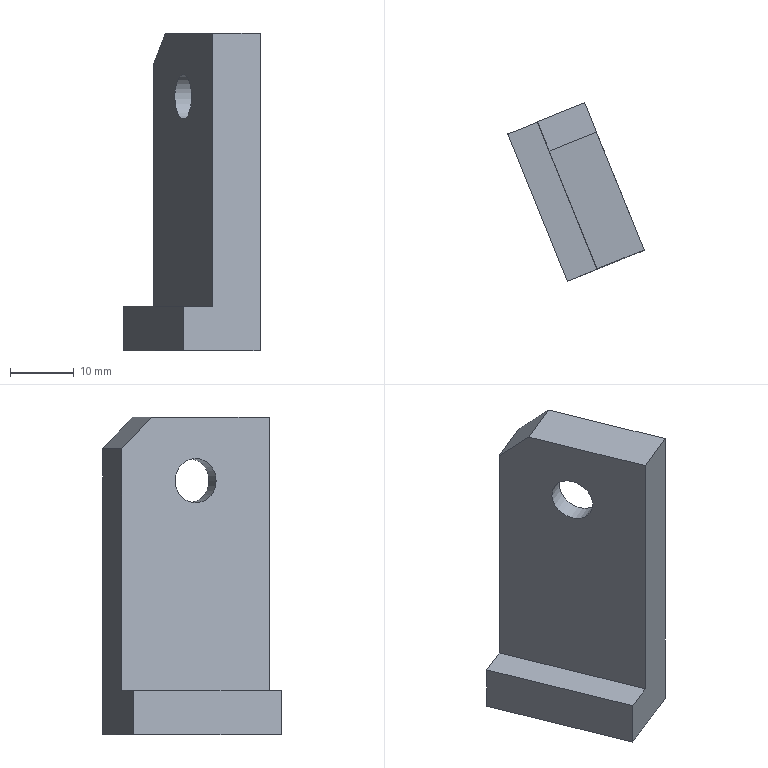Part | NX | features solid 2 | 1 solid | 12 faces | box 21.419 x 28.049 x 50 mm | volume 9656 mm3 | plane 10 | spline 2
STEP:
#1=CARTESIAN_POINT('',(-700.084,400.509,62.979));
#2=VERTEX_POINT('',#1);
#3=CARTESIAN_POINT('',(-699.783,399.764,61.255));
#4=CARTESIAN_POINT('',(-700.385,401.254,64.703));
#5=CARTESIAN_POINT('',(-701.18,403.223,65.476));
#6=CARTESIAN_POINT('',(-702.472,406.42,63.868));
#7=CARTESIAN_POINT('',(-702.761,407.136,61.745));
#8=CARTESIAN_POINT('',(-702.159,405.646,58.297));
#9=CARTESIAN_POINT('',(-701.364,403.677,57.524));
#10=CARTESIAN_POINT('',(-700.072,400.48,59.132));
#11=CARTESIAN_POINT('',(-699.783,399.764,61.255));
#12=CARTESIAN_POINT('',(-700.385,401.254,64.703));
#13=B_SPLINE_CURVE_WITH_KNOTS('',3,(#3,#4,#5,#6,#7,#8,#9,#10,#11,#12),.UNSPECIFIED.,.T.,.F.,(2,2,2,2,2,2,2),(-0.25,0.,0.25,0.5,0.75,1.,1.25),.UNSPECIFIED.);
#14=EDGE_CURVE('',#2,#2,#13,.T.);
#15=ORIENTED_EDGE('',*,*,#14,.F.);
#16=EDGE_LOOP('',(#15));
#17=FACE_BOUND('',#16,.T.);
#18=CARTESIAN_POINT('',(-705.955,415.04,28.5));
#19=VERTEX_POINT('',#18);
#20=CARTESIAN_POINT('',(-696.589,391.86,28.5));
#21=VERTEX_POINT('',#20);
#22=CARTESIAN_POINT('',(-696.589,391.86,28.5));
#23=DIRECTION('',(0.3746,-0.9272,0.000000023));
#24=VECTOR('',#23,1000.);
#25=LINE('',#22,#24);
#26=EDGE_CURVE('',#19,#21,#25,.T.);
#27=ORIENTED_EDGE('',*,*,#26,.T.);
#28=CARTESIAN_POINT('',(-696.589,391.86,71.5));
#29=VERTEX_POINT('',#28);
#30=CARTESIAN_POINT('',(-696.589,391.86,21.5));
#31=DIRECTION('',(0.,0.,1.));
#32=VECTOR('',#31,1000.);
#33=LINE('',#30,#32);
#34=EDGE_CURVE('',#21,#29,#33,.T.);
#35=ORIENTED_EDGE('',*,*,#34,.T.);
#36=CARTESIAN_POINT('',(-704.082,410.404,71.5));
#37=VERTEX_POINT('',#36);
#38=CARTESIAN_POINT('',(-696.589,391.86,71.5));
#39=DIRECTION('',(-0.3746,0.9272,0.));
#40=VECTOR('',#39,1000.);
#41=LINE('',#38,#40);
#42=EDGE_CURVE('',#29,#37,#41,.T.);
#43=ORIENTED_EDGE('',*,*,#42,.T.);
#44=CARTESIAN_POINT('',(-705.955,415.04,66.5));
#45=VERTEX_POINT('',#44);
#46=CARTESIAN_POINT('',(-705.955,415.04,66.5));
#47=DIRECTION('',(0.2649,-0.6556,0.7071));
#48=VECTOR('',#47,1000.);
#49=LINE('',#46,#48);
#50=EDGE_CURVE('',#45,#37,#49,.T.);
#51=ORIENTED_EDGE('',*,*,#50,.F.);
#52=CARTESIAN_POINT('',(-705.955,415.04,51.5));
#53=DIRECTION('',(0.,0.,1.));
#54=VECTOR('',#53,1000.);
#55=LINE('',#52,#54);
#56=EDGE_CURVE('',#19,#45,#55,.T.);
#57=ORIENTED_EDGE('',*,*,#56,.F.);
#58=EDGE_LOOP('',(#27,#35,#43,#51,#57));
#59=FACE_BOUND('',#58,.T.);
#60=CARTESIAN_POINT('',(-696.589,391.86,91.5));
#61=DIRECTION('',(0.9272,0.3746,0.));
#62=DIRECTION('',(0.3244,-0.803,0.5));
#63=AXIS2_PLACEMENT_3D('',#60,#61,#62);
#64=PLANE('',#63);
#65=ADVANCED_FACE('',(#17,#59),#64,.F.);
#66=CARTESIAN_POINT('',(-698.537,418.037,66.5));
#67=VERTEX_POINT('',#66);
#68=CARTESIAN_POINT('',(-696.664,413.401,71.5));
#69=VERTEX_POINT('',#68);
#70=CARTESIAN_POINT('',(-698.537,418.037,66.5));
#71=DIRECTION('',(0.2649,-0.6556,0.7071));
#72=VECTOR('',#71,1000.);
#73=LINE('',#70,#72);
#74=EDGE_CURVE('',#67,#69,#73,.T.);
#75=ORIENTED_EDGE('',*,*,#74,.F.);
#76=CARTESIAN_POINT('',(-705.955,415.04,66.5));
#77=DIRECTION('',(0.9272,0.3746,0.));
#78=VECTOR('',#77,1000.);
#79=LINE('',#76,#78);
#80=EDGE_CURVE('',#45,#67,#79,.T.);
#81=ORIENTED_EDGE('',*,*,#80,.F.);
#82=ORIENTED_EDGE('',*,*,#50,.T.);
#83=CARTESIAN_POINT('',(-704.082,410.404,71.5));
#84=DIRECTION('',(0.9272,0.3746,0.));
#85=VECTOR('',#84,1000.);
#86=LINE('',#83,#85);
#87=EDGE_CURVE('',#37,#69,#86,.T.);
#88=ORIENTED_EDGE('',*,*,#87,.T.);
#89=EDGE_LOOP('',(#75,#81,#82,#88));
#90=FACE_BOUND('',#89,.T.);
#91=CARTESIAN_POINT('',(-705.955,415.04,66.5));
#92=DIRECTION('',(0.2649,-0.6556,-0.7071));
#93=DIRECTION('',(0.2649,-0.6556,0.7071));
#94=AXIS2_PLACEMENT_3D('',#91,#92,#93);
#95=PLANE('',#94);
#96=ADVANCED_FACE('',(#90),#95,.F.);
#97=CARTESIAN_POINT('',(-689.172,394.857,71.5));
#98=VERTEX_POINT('',#97);
#99=CARTESIAN_POINT('',(-689.172,394.857,71.5));
#100=DIRECTION('',(-0.3746,0.9272,0.));
#101=VECTOR('',#100,1000.);
#102=LINE('',#99,#101);
#103=EDGE_CURVE('',#98,#69,#102,.T.);
#104=ORIENTED_EDGE('',*,*,#103,.T.);
#105=ORIENTED_EDGE('',*,*,#87,.F.);
#106=ORIENTED_EDGE('',*,*,#42,.F.);
#107=CARTESIAN_POINT('',(-696.589,391.86,71.5));
#108=DIRECTION('',(0.9272,0.3746,0.));
#109=VECTOR('',#108,1000.);
#110=LINE('',#107,#109);
#111=EDGE_CURVE('',#29,#98,#110,.T.);
#112=ORIENTED_EDGE('',*,*,#111,.T.);
#113=EDGE_LOOP('',(#104,#105,#106,#112));
#114=FACE_BOUND('',#113,.T.);
#115=CARTESIAN_POINT('',(-696.589,391.86,71.5));
#116=DIRECTION('',(0.,0.,1.));
#117=DIRECTION('',(-0.3746,0.9272,0.));
#118=AXIS2_PLACEMENT_3D('',#115,#116,#117);
#119=PLANE('',#118);
#120=ADVANCED_FACE('',(#114),#119,.T.);
#121=CARTESIAN_POINT('',(-689.172,394.857,21.5));
#122=VERTEX_POINT('',#121);
#123=CARTESIAN_POINT('',(-689.172,394.857,21.5));
#124=DIRECTION('',(0.,0.,1.));
#125=VECTOR('',#124,1000.);
#126=LINE('',#123,#125);
#127=EDGE_CURVE('',#122,#98,#126,.T.);
#128=ORIENTED_EDGE('',*,*,#127,.T.);
#129=ORIENTED_EDGE('',*,*,#111,.F.);
#130=ORIENTED_EDGE('',*,*,#34,.F.);
#131=CARTESIAN_POINT('',(-701.225,389.987,28.5));
#132=VERTEX_POINT('',#131);
#133=CARTESIAN_POINT('',(-701.225,389.987,28.5));
#134=DIRECTION('',(0.9272,0.3746,0.));
#135=VECTOR('',#134,1000.);
#136=LINE('',#133,#135);
#137=EDGE_CURVE('',#132,#21,#136,.T.);
#138=ORIENTED_EDGE('',*,*,#137,.F.);
#139=CARTESIAN_POINT('',(-701.225,389.987,21.5));
#140=VERTEX_POINT('',#139);
#141=CARTESIAN_POINT('',(-701.225,389.987,31.5));
#142=DIRECTION('',(0.,0.,-1.));
#143=VECTOR('',#142,1000.);
#144=LINE('',#141,#143);
#145=EDGE_CURVE('',#132,#140,#144,.T.);
#146=ORIENTED_EDGE('',*,*,#145,.T.);
#147=CARTESIAN_POINT('',(-696.589,391.86,21.5));
#148=DIRECTION('',(0.9272,0.3746,0.));
#149=VECTOR('',#148,1000.);
#150=LINE('',#147,#149);
#151=EDGE_CURVE('',#140,#122,#150,.T.);
#152=ORIENTED_EDGE('',*,*,#151,.T.);
#153=EDGE_LOOP('',(#128,#129,#130,#138,#146,#152));
#154=FACE_BOUND('',#153,.T.);
#155=CARTESIAN_POINT('',(-696.589,391.86,21.5));
#156=DIRECTION('',(0.3746,-0.9272,0.));
#157=DIRECTION('',(0.,0.,1.));
#158=AXIS2_PLACEMENT_3D('',#155,#156,#157);
#159=PLANE('',#158);
#160=ADVANCED_FACE('',(#154),#159,.T.);
#161=CARTESIAN_POINT('',(-698.537,418.037,21.5));
#162=VERTEX_POINT('',#161);
#163=CARTESIAN_POINT('',(-698.537,418.037,21.5));
#164=DIRECTION('',(0.3746,-0.9272,0.));
#165=VECTOR('',#164,1000.);
#166=LINE('',#163,#165);
#167=EDGE_CURVE('',#162,#122,#166,.T.);
#168=ORIENTED_EDGE('',*,*,#167,.T.);
#169=ORIENTED_EDGE('',*,*,#151,.F.);
#170=CARTESIAN_POINT('',(-710.591,413.167,21.5));
#171=VERTEX_POINT('',#170);
#172=CARTESIAN_POINT('',(-710.591,413.167,21.5));
#173=DIRECTION('',(0.3746,-0.9272,0.));
#174=VECTOR('',#173,1000.);
#175=LINE('',#172,#174);
#176=EDGE_CURVE('',#171,#140,#175,.T.);
#177=ORIENTED_EDGE('',*,*,#176,.F.);
#178=CARTESIAN_POINT('',(-705.955,415.04,21.5));
#179=DIRECTION('',(0.9272,0.3746,0.));
#180=VECTOR('',#179,1000.);
#181=LINE('',#178,#180);
#182=EDGE_CURVE('',#171,#162,#181,.T.);
#183=ORIENTED_EDGE('',*,*,#182,.T.);
#184=EDGE_LOOP('',(#168,#169,#177,#183));
#185=FACE_BOUND('',#184,.T.);
#186=CARTESIAN_POINT('',(-705.955,415.04,21.5));
#187=DIRECTION('',(0.,0.,-1.));
#188=DIRECTION('',(0.3746,-0.9272,0.));
#189=AXIS2_PLACEMENT_3D('',#186,#187,#188);
#190=PLANE('',#189);
#191=ADVANCED_FACE('',(#185),#190,.T.);
#192=CARTESIAN_POINT('',(-698.537,418.037,51.5));
#193=DIRECTION('',(0.,0.,1.));
#194=VECTOR('',#193,1000.);
#195=LINE('',#192,#194);
#196=EDGE_CURVE('',#162,#67,#195,.T.);
#197=ORIENTED_EDGE('',*,*,#196,.F.);
#198=ORIENTED_EDGE('',*,*,#182,.F.);
#199=CARTESIAN_POINT('',(-710.591,413.167,28.5));
#200=VERTEX_POINT('',#199);
#201=CARTESIAN_POINT('',(-710.591,413.167,31.5));
#202=DIRECTION('',(0.,0.,-1.));
#203=VECTOR('',#202,1000.);
#204=LINE('',#201,#203);
#205=EDGE_CURVE('',#200,#171,#204,.T.);
#206=ORIENTED_EDGE('',*,*,#205,.F.);
#207=CARTESIAN_POINT('',(-710.591,413.167,28.5));
#208=DIRECTION('',(0.9272,0.3746,0.));
#209=VECTOR('',#208,1000.);
#210=LINE('',#207,#209);
#211=EDGE_CURVE('',#200,#19,#210,.T.);
#212=ORIENTED_EDGE('',*,*,#211,.T.);
#213=ORIENTED_EDGE('',*,*,#56,.T.);
#214=ORIENTED_EDGE('',*,*,#80,.T.);
#215=EDGE_LOOP('',(#197,#198,#206,#212,#213,#214));
#216=FACE_BOUND('',#215,.T.);
#217=CARTESIAN_POINT('',(-705.955,415.04,51.5));
#218=DIRECTION('',(0.3746,-0.9272,0.));
#219=DIRECTION('',(0.,0.,1.));
#220=AXIS2_PLACEMENT_3D('',#217,#218,#219);
#221=PLANE('',#220);
#222=ADVANCED_FACE('',(#216),#221,.F.);
#223=CARTESIAN_POINT('',(-691.139,399.724,64.881));
#224=VERTEX_POINT('',#223);
#225=CARTESIAN_POINT('',(-690.805,398.899,62.971));
#226=CARTESIAN_POINT('',(-691.472,400.55,66.79));
#227=CARTESIAN_POINT('',(-692.088,402.074,68.297));
#228=CARTESIAN_POINT('',(-693.571,405.746,69.738));
#229=CARTESIAN_POINT('',(-694.406,407.811,69.641));
#230=CARTESIAN_POINT('',(-695.836,411.352,67.86));
#231=CARTESIAN_POINT('',(-696.401,412.749,66.216));
#232=CARTESIAN_POINT('',(-696.941,414.085,62.256));
#233=CARTESIAN_POINT('',(-696.904,413.995,60.029));
#234=CARTESIAN_POINT('',(-696.237,412.344,56.21));
#235=CARTESIAN_POINT('',(-695.621,410.819,54.703));
#236=CARTESIAN_POINT('',(-694.138,407.148,53.262));
#237=CARTESIAN_POINT('',(-693.303,405.083,53.359));
#238=CARTESIAN_POINT('',(-691.873,401.542,55.14));
#239=CARTESIAN_POINT('',(-691.308,400.145,56.784));
#240=CARTESIAN_POINT('',(-690.769,398.809,60.744));
#241=CARTESIAN_POINT('',(-690.805,398.899,62.971));
#242=CARTESIAN_POINT('',(-691.472,400.55,66.79));
#243=B_SPLINE_CURVE_WITH_KNOTS('',3,(#225,#226,#227,#228,#229,#230,#231,#232,#233,#234,#235,#236,#237,#238,#239,#240,#241,#242),.UNSPECIFIED.,.T.,.F.,(2,2,2,2,2,2,2,2,2,2,2),(-0.125,0.,0.125,0.25,0.375,0.5,0.625,0.75,0.875,1.,1.125),.UNSPECIFIED.);
#244=EDGE_CURVE('',#224,#224,#243,.T.);
#245=ORIENTED_EDGE('',*,*,#244,.T.);
#246=EDGE_LOOP('',(#245));
#247=FACE_BOUND('',#246,.T.);
#248=ORIENTED_EDGE('',*,*,#74,.T.);
#249=ORIENTED_EDGE('',*,*,#103,.F.);
#250=ORIENTED_EDGE('',*,*,#127,.F.);
#251=ORIENTED_EDGE('',*,*,#167,.F.);
#252=ORIENTED_EDGE('',*,*,#196,.T.);
#253=EDGE_LOOP('',(#248,#249,#250,#251,#252));
#254=FACE_BOUND('',#253,.T.);
#255=CARTESIAN_POINT('',(-689.172,394.857,91.5));
#256=DIRECTION('',(0.9272,0.3746,0.));
#257=DIRECTION('',(0.3244,-0.803,0.5));
#258=AXIS2_PLACEMENT_3D('',#255,#256,#257);
#259=PLANE('',#258);
#260=ADVANCED_FACE('',(#247,#254),#259,.T.);
#261=CARTESIAN_POINT('',(-695.774,397.851,64.881));
#262=VERTEX_POINT('',#261);
#263=CARTESIAN_POINT('',(-695.441,397.026,62.971));
#264=CARTESIAN_POINT('',(-696.108,398.677,66.79));
#265=CARTESIAN_POINT('',(-696.724,400.201,68.297));
#266=CARTESIAN_POINT('',(-698.207,403.873,69.738));
#267=CARTESIAN_POINT('',(-699.042,405.938,69.641));
#268=CARTESIAN_POINT('',(-700.472,409.479,67.86));
#269=CARTESIAN_POINT('',(-701.037,410.876,66.216));
#270=CARTESIAN_POINT('',(-701.577,412.212,62.256));
#271=CARTESIAN_POINT('',(-701.54,412.122,60.029));
#272=CARTESIAN_POINT('',(-700.873,410.471,56.21));
#273=CARTESIAN_POINT('',(-700.257,408.946,54.703));
#274=CARTESIAN_POINT('',(-698.774,405.275,53.262));
#275=CARTESIAN_POINT('',(-697.939,403.21,53.359));
#276=CARTESIAN_POINT('',(-696.509,399.669,55.14));
#277=CARTESIAN_POINT('',(-695.944,398.272,56.784));
#278=CARTESIAN_POINT('',(-695.404,396.936,60.744));
#279=CARTESIAN_POINT('',(-695.441,397.026,62.971));
#280=CARTESIAN_POINT('',(-696.108,398.677,66.79));
#281=B_SPLINE_CURVE_WITH_KNOTS('',3,(#263,#264,#265,#266,#267,#268,#269,#270,#271,#272,#273,#274,#275,#276,#277,#278,#279,#280),.UNSPECIFIED.,.T.,.F.,(2,2,2,2,2,2,2,2,2,2,2),(-0.125,0.,0.125,0.25,0.375,0.5,0.625,0.75,0.875,1.,1.125),.UNSPECIFIED.);
#282=EDGE_CURVE('',#262,#262,#281,.T.);
#283=ORIENTED_EDGE('',*,*,#282,.T.);
#284=EDGE_LOOP('',(#283));
#285=FACE_BOUND('',#284,.T.);
#286=ORIENTED_EDGE('',*,*,#244,.F.);
#287=EDGE_LOOP('',(#286));
#288=FACE_BOUND('',#287,.T.);
#289=CARTESIAN_POINT('',(-695.37,396.85,58.468));
#290=CARTESIAN_POINT('',(-690.734,398.723,58.468));
#291=CARTESIAN_POINT('',(-695.481,397.124,65.247));
#292=CARTESIAN_POINT('',(-690.845,398.997,65.247));
#293=CARTESIAN_POINT('',(-697.355,401.762,69.831));
#294=CARTESIAN_POINT('',(-692.719,403.635,69.831));
#295=CARTESIAN_POINT('',(-699.894,408.048,69.535));
#296=CARTESIAN_POINT('',(-695.258,409.921,69.535));
#297=CARTESIAN_POINT('',(-701.611,412.298,64.532));
#298=CARTESIAN_POINT('',(-696.975,414.171,64.532));
#299=CARTESIAN_POINT('',(-701.5,412.024,57.753));
#300=CARTESIAN_POINT('',(-696.865,413.897,57.753));
#301=CARTESIAN_POINT('',(-699.626,407.385,53.169));
#302=CARTESIAN_POINT('',(-694.99,409.258,53.169));
#303=CARTESIAN_POINT('',(-697.087,401.1,53.465));
#304=CARTESIAN_POINT('',(-692.451,402.973,53.465));
#305=CARTESIAN_POINT('',(-695.37,396.85,58.468));
#306=CARTESIAN_POINT('',(-690.734,398.723,58.468));
#307=CARTESIAN_POINT('',(-695.481,397.124,65.247));
#308=CARTESIAN_POINT('',(-690.845,398.997,65.247));
#309=CARTESIAN_POINT('',(-697.355,401.762,69.831));
#310=CARTESIAN_POINT('',(-692.719,403.635,69.831));
#311=B_SPLINE_SURFACE_WITH_KNOTS('',3,1,((#289,#290),(#291,#292),(#293,#294),(#295,#296),(#297,#298),(#299,#300),(#301,#302),(#303,#304),(#305,#306),(#307,#308),(#309,#310)),.SURF_OF_LINEAR_EXTRUSION.,.T.,.F.,.F.,(1,1,1,1,1,1,1,1,1,1,1,1,1,1,1),(2,2),(-0.375,-0.25,-0.125,0.,0.125,0.25,0.375,0.5,0.625,0.75,0.875,1.,1.125,1.25,1.375),(0.,1.),.UNSPECIFIED.);
#312=ADVANCED_FACE('',(#285,#288),#311,.T.);
#313=CARTESIAN_POINT('',(-697.302,401.633,62.979));
#314=VERTEX_POINT('',#313);
#315=CARTESIAN_POINT('',(-697.001,400.887,61.255));
#316=CARTESIAN_POINT('',(-697.603,402.378,64.703));
#317=CARTESIAN_POINT('',(-698.399,404.347,65.476));
#318=CARTESIAN_POINT('',(-699.69,407.544,63.868));
#319=CARTESIAN_POINT('',(-699.98,408.26,61.745));
#320=CARTESIAN_POINT('',(-699.378,406.77,58.297));
#321=CARTESIAN_POINT('',(-698.582,404.801,57.524));
#322=CARTESIAN_POINT('',(-697.291,401.604,59.132));
#323=CARTESIAN_POINT('',(-697.001,400.887,61.255));
#324=CARTESIAN_POINT('',(-697.603,402.378,64.703));
#325=B_SPLINE_CURVE_WITH_KNOTS('',3,(#315,#316,#317,#318,#319,#320,#321,#322,#323,#324),.UNSPECIFIED.,.T.,.F.,(2,2,2,2,2,2,2),(-0.25,0.,0.25,0.5,0.75,1.,1.25),.UNSPECIFIED.);
#326=EDGE_CURVE('',#314,#314,#325,.F.);
#327=ORIENTED_EDGE('',*,*,#326,.F.);
#328=EDGE_LOOP('',(#327));
#329=FACE_BOUND('',#328,.T.);
#330=ORIENTED_EDGE('',*,*,#282,.F.);
#331=EDGE_LOOP('',(#330));
#332=FACE_BOUND('',#331,.T.);
#333=CARTESIAN_POINT('',(-701.207,411.296,58.119));
#334=DIRECTION('',(-0.9272,-0.3746,0.));
#335=DIRECTION('',(-0.3244,0.803,-0.5));
#336=AXIS2_PLACEMENT_3D('',#333,#334,#335);
#337=PLANE('',#336);
#338=ADVANCED_FACE('',(#329,#332),#337,.F.);
#339=ORIENTED_EDGE('',*,*,#14,.T.);
#340=EDGE_LOOP('',(#339));
#341=FACE_BOUND('',#340,.T.);
#342=ORIENTED_EDGE('',*,*,#326,.T.);
#343=EDGE_LOOP('',(#342));
#344=FACE_BOUND('',#343,.T.);
#345=CARTESIAN_POINT('',(-699.917,400.095,60.183));
#346=CARTESIAN_POINT('',(-697.135,401.219,60.183));
#347=CARTESIAN_POINT('',(-699.952,400.182,63.143));
#348=CARTESIAN_POINT('',(-697.17,401.306,63.143));
#349=CARTESIAN_POINT('',(-700.779,402.229,65.118));
#350=CARTESIAN_POINT('',(-697.997,403.353,65.118));
#351=CARTESIAN_POINT('',(-701.888,404.974,65.024));
#352=CARTESIAN_POINT('',(-699.106,406.098,65.024));
#353=CARTESIAN_POINT('',(-702.628,406.805,62.817));
#354=CARTESIAN_POINT('',(-699.846,407.929,62.817));
#355=CARTESIAN_POINT('',(-702.592,406.718,59.857));
#356=CARTESIAN_POINT('',(-699.811,407.841,59.857));
#357=CARTESIAN_POINT('',(-701.765,404.671,57.882));
#358=CARTESIAN_POINT('',(-698.984,405.795,57.882));
#359=CARTESIAN_POINT('',(-700.656,401.926,57.976));
#360=CARTESIAN_POINT('',(-697.875,403.05,57.976));
#361=CARTESIAN_POINT('',(-699.917,400.095,60.183));
#362=CARTESIAN_POINT('',(-697.135,401.219,60.183));
#363=CARTESIAN_POINT('',(-699.952,400.182,63.143));
#364=CARTESIAN_POINT('',(-697.17,401.306,63.143));
#365=CARTESIAN_POINT('',(-700.779,402.229,65.118));
#366=CARTESIAN_POINT('',(-697.997,403.353,65.118));
#367=B_SPLINE_SURFACE_WITH_KNOTS('',3,1,((#345,#346),(#347,#348),(#349,#350),(#351,#352),(#353,#354),(#355,#356),(#357,#358),(#359,#360),(#361,#362),(#363,#364),(#365,#366)),.SURF_OF_LINEAR_EXTRUSION.,.T.,.F.,.F.,(1,1,1,1,1,1,1,1,1,1,1,1,1,1,1),(2,2),(-0.375,-0.25,-0.125,0.,0.125,0.25,0.375,0.5,0.625,0.75,0.875,1.,1.125,1.25,1.375),(0.,1.),.UNSPECIFIED.);
#368=ADVANCED_FACE('',(#341,#344),#367,.T.);
#369=ORIENTED_EDGE('',*,*,#26,.F.);
#370=ORIENTED_EDGE('',*,*,#211,.F.);
#371=CARTESIAN_POINT('',(-710.591,413.167,28.5));
#372=DIRECTION('',(0.3746,-0.9272,0.000000023));
#373=VECTOR('',#372,1000.);
#374=LINE('',#371,#373);
#375=EDGE_CURVE('',#200,#132,#374,.T.);
#376=ORIENTED_EDGE('',*,*,#375,.T.);
#377=ORIENTED_EDGE('',*,*,#137,.T.);
#378=EDGE_LOOP('',(#369,#370,#376,#377));
#379=FACE_BOUND('',#378,.T.);
#380=CARTESIAN_POINT('',(-710.591,413.167,28.5));
#381=DIRECTION('',(0.000000009,-0.000000021,-1.));
#382=DIRECTION('',(0.3746,-0.9272,0.000000023));
#383=AXIS2_PLACEMENT_3D('',#380,#381,#382);
#384=PLANE('',#383);
#385=ADVANCED_FACE('',(#379),#384,.F.);
#386=ORIENTED_EDGE('',*,*,#176,.T.);
#387=ORIENTED_EDGE('',*,*,#145,.F.);
#388=ORIENTED_EDGE('',*,*,#375,.F.);
#389=ORIENTED_EDGE('',*,*,#205,.T.);
#390=EDGE_LOOP('',(#386,#387,#388,#389));
#391=FACE_BOUND('',#390,.T.);
#392=CARTESIAN_POINT('',(-710.591,413.167,21.5));
#393=DIRECTION('',(0.9272,0.3746,0.));
#394=DIRECTION('',(0.3244,-0.803,0.5));
#395=AXIS2_PLACEMENT_3D('',#392,#393,#394);
#396=PLANE('',#395);
#397=ADVANCED_FACE('',(#391),#396,.F.);
#398=CLOSED_SHELL('',(#65,#96,#120,#160,#191,#222,#260,#312,#338,#368,#385,#397));
#399=MANIFOLD_SOLID_BREP('',#398);
#400=(LENGTH_UNIT()NAMED_UNIT(*)SI_UNIT(.MILLI.,.METRE.));
#401=UNCERTAINTY_MEASURE_WITH_UNIT(LENGTH_MEASURE(0.0508),#400,'','');
#402=(NAMED_UNIT(*)PLANE_ANGLE_UNIT()SI_UNIT($,.RADIAN.));
#403=(NAMED_UNIT(*)SI_UNIT($,.STERADIAN.)SOLID_ANGLE_UNIT());
#404=(GEOMETRIC_REPRESENTATION_CONTEXT(3)GLOBAL_UNCERTAINTY_ASSIGNED_CONTEXT((#401))GLOBAL_UNIT_ASSIGNED_CONTEXT((#400,#402,#403))REPRESENTATION_CONTEXT('',''));
#405=ADVANCED_BREP_SHAPE_REPRESENTATION('',(#399),#404);